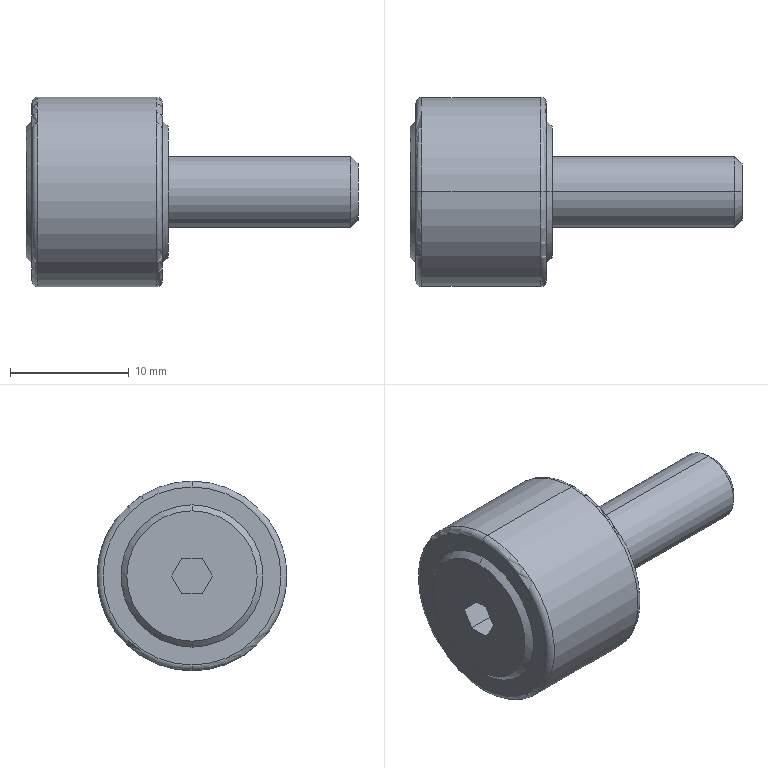Part | STEP file | CFA6_16body | 1 solid | 26 faces | box 28 x 16 x 16 mm | volume 2741 mm3 | plane 12 | cone 6 | cylinder 4 | torus 4 | commonest cylinder face diameters 6 x2 16 x2